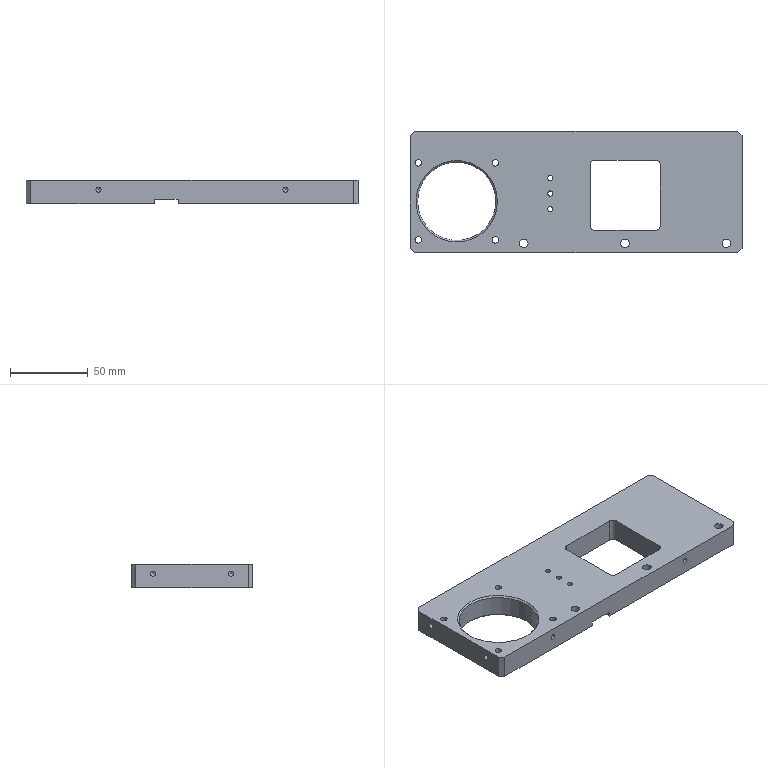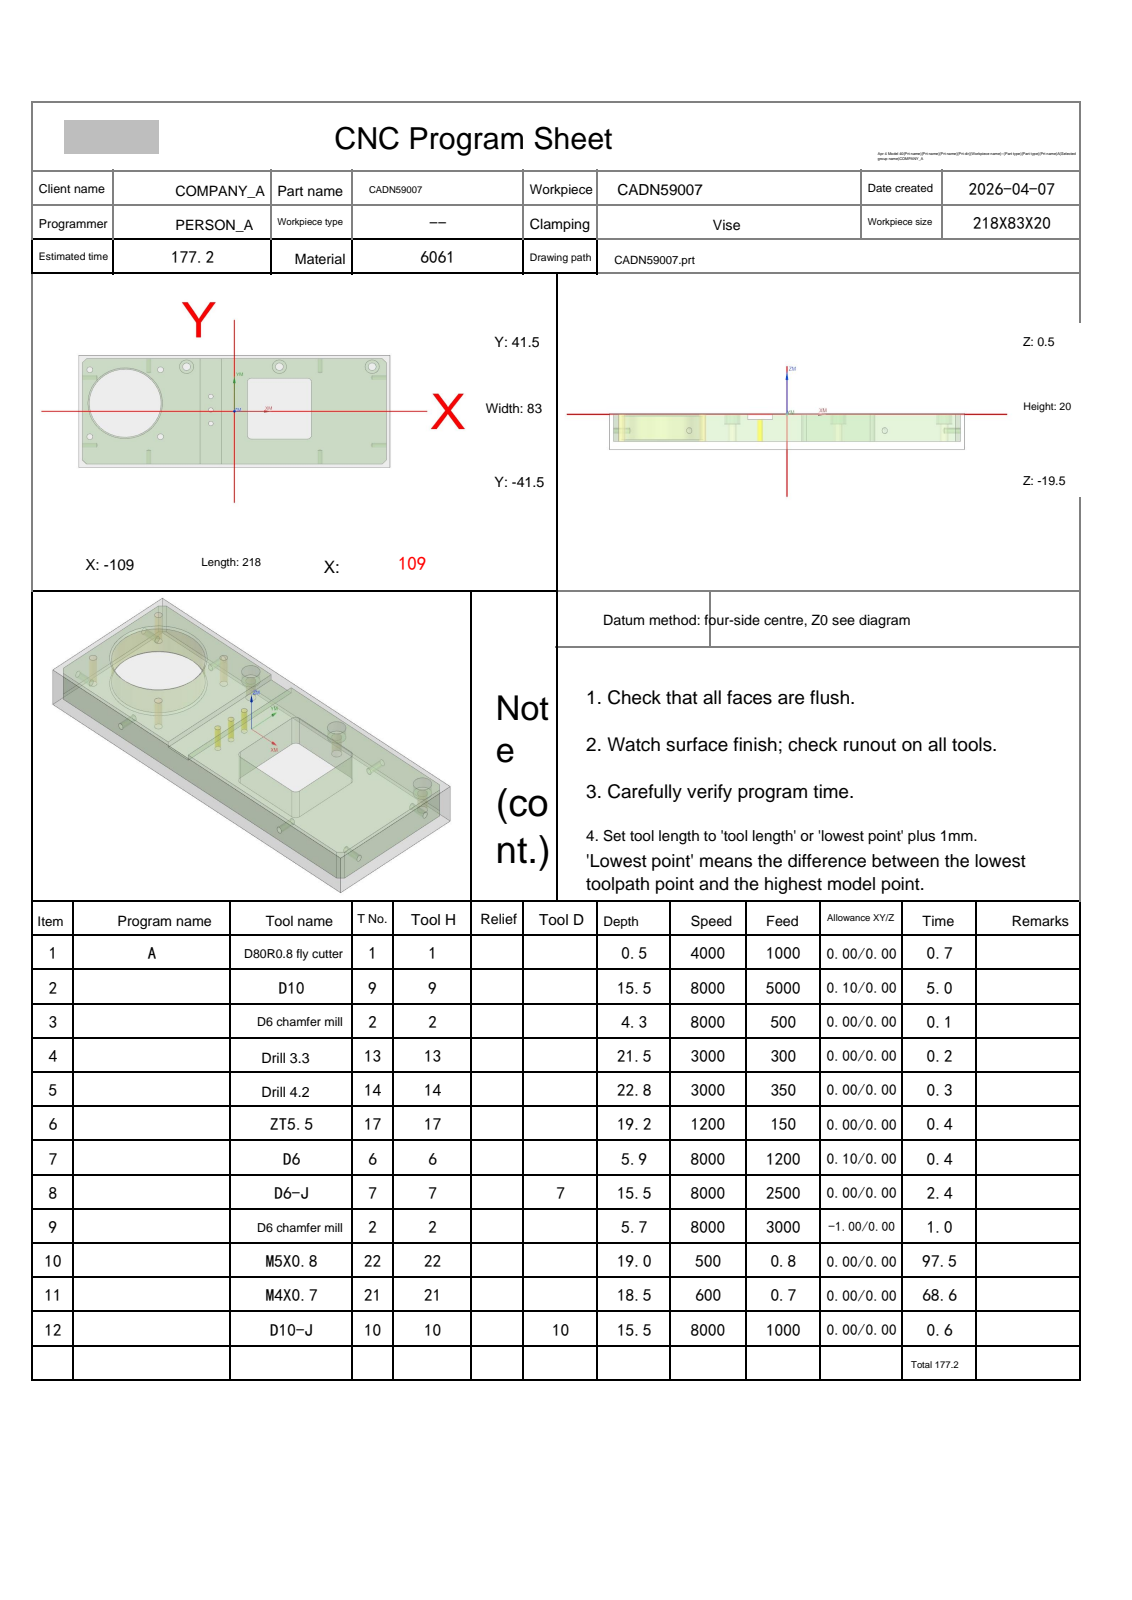NC program | NX | posted by the shop | part box 213 x 78 x 15 mm
Lines 1 to 890 of 7501:
%
O0001
(Machine time: 336.47 MIN)
(===Total Tool:11===)
(T1=D80R0.8 fly cutter D=80.  R=0.8  D-  H01 Z=0.    )
(T9=D10     D=10.  R=0.   D-  H09 Z=-15.  )
(T2=D6 chamfer mill   D=6.   R=0.   D-  H02 Z=-5.2  )
(T13=Drill 3.3  D=3.3  DR_a=118 D-  H13 Z=-20.99)
(T14=Drill 4.2  D=4.2  DR_a=118 D-  H14 Z=-22.26)
(T17=ZT5.5  D=5.5  DR_a=118 D-  H17 Z=-18.65)
(T6=D6      D=6.   R=0.   D-  H06 Z=-5.4  )
(T7=D6-J    D=6.   R=0.   D7  H07 Z=-15.  )
(T22=M5X0.8 D=4.2  DR_a=180 D-  H22 Z=-18.5 )
(T21=M4X0.7 D=3.3  DR_a=180 D-  H21 Z=-18.  )
(T10=D10-J  D=10.  R=0.   D10 H10 Z=-15.  )
G80 G90 G17 G49 G40
G91 G28 Z0
M01
N1 T01 M06
(D80R0.8 fly cutter  D=80. R=0.8 H=01 ce=0.00 di=0.00)
G00 G90 G54 X151.5 Y-26.333 M03 S4000
G43 H01 Z20.
M08
Z2.
G01 Z0.0 F1000.
X146.5
X-146.5
Y26.333
X146.5
X151.5
Z2.
G00 Z20.
G91 G28 Z0.0
M05
M09
G91 G28 Z0.0
M01
N2 T09 M06
(D10  D=10. R=0. H=09 ce=0.10 di=0.00)
G00 G90 G54 X0.0 Y44.1 M03 S8000
G43 H09 Z20.
M08
Z.5
G01 X103.5 Z.368 F5000.
G02 X107.106 Y42.606 Z.363 I0.0 J-5.1
G01 X110.106 Y39.606 Z.357
G02 X111.6 Y36. Z.352 I-3.606 J-3.606
G01 Y-36. Z.26
G02 X110.106 Y-39.606 Z.255 I-5.1 J0.0
G01 X107.106 Y-42.606 Z.25
G02 X103.5 Y-44.1 Z.245 I-3.606 J3.606
G01 X-103.5 Z-.02
G02 X-107.106 Y-42.606 Z-.025 I0.0 J5.1
G01 X-110.106 Y-39.606 Z-.03
G02 X-111.6 Y-36. Z-.035 I3.606 J3.606
G01 Y36. Z-.127
G02 X-110.106 Y39.606 Z-.132 I5.1 J0.0
G01 X-107.106 Y42.606 Z-.138
G02 X-103.5 Y44.1 Z-.143 I3.606 J-3.606
G01 X103.5 Z-.407
G02 X107.106 Y42.606 Z-.412 I0.0 J-5.1
G01 X110.106 Y39.606 Z-.418
G02 X111.6 Y36. Z-.423 I-3.606 J-3.606
G01 Y-36. Z-.515
G02 X110.106 Y-39.606 Z-.52 I-5.1 J0.0
G01 X107.106 Y-42.606 Z-.525
G02 X103.5 Y-44.1 Z-.53 I-3.606 J3.606
G01 X-103.5 Z-.795
G02 X-107.106 Y-42.606 Z-.8 I0.0 J5.1
G01 X-110.106 Y-39.606 Z-.805
G02 X-111.6 Y-36. Z-.81 I3.606 J3.606
G01 Y36. Z-.902
G02 X-110.106 Y39.606 Z-.907 I5.1 J0.0
G01 X-107.106 Y42.606 Z-.913
G02 X-103.5 Y44.1 Z-.918 I3.606 J-3.606
G01 X103.5 Z-1.182
G02 X107.106 Y42.606 Z-1.187 I0.0 J-5.1
G01 X110.106 Y39.606 Z-1.193
G02 X111.6 Y36. Z-1.198 I-3.606 J-3.606
G01 Y-36. Z-1.29
G02 X110.106 Y-39.606 Z-1.295 I-5.1 J0.0
G01 X107.106 Y-42.606 Z-1.3
G02 X103.5 Y-44.1 Z-1.305 I-3.606 J3.606
G01 X-103.5 Z-1.57
G02 X-107.106 Y-42.606 Z-1.575 I0.0 J5.1
G01 X-110.106 Y-39.606 Z-1.58
G02 X-111.6 Y-36. Z-1.585 I3.606 J3.606
G01 Y36. Z-1.677
G02 X-110.106 Y39.606 Z-1.682 I5.1 J0.0
G01 X-107.106 Y42.606 Z-1.688
G02 X-103.5 Y44.1 Z-1.693 I3.606 J-3.606
G01 X103.5 Z-1.957
G02 X107.106 Y42.606 Z-1.962 I0.0 J-5.1
G01 X110.106 Y39.606 Z-1.968
G02 X111.6 Y36. Z-1.973 I-3.606 J-3.606
G01 Y-36. Z-2.065
G02 X110.106 Y-39.606 Z-2.07 I-5.1 J0.0
G01 X107.106 Y-42.606 Z-2.075
G02 X103.5 Y-44.1 Z-2.08 I-3.606 J3.606
G01 X-103.5 Z-2.345
G02 X-107.106 Y-42.606 Z-2.35 I0.0 J5.1
G01 X-110.106 Y-39.606 Z-2.355
G02 X-111.6 Y-36. Z-2.36 I3.606 J3.606
G01 Y36. Z-2.452
G02 X-110.106 Y39.606 Z-2.457 I5.1 J0.0
G01 X-107.106 Y42.606 Z-2.463
G02 X-103.5 Y44.1 Z-2.468 I3.606 J-3.606
G01 X103.5 Z-2.732
G02 X107.106 Y42.606 Z-2.737 I0.0 J-5.1
G01 X110.106 Y39.606 Z-2.743
G02 X111.6 Y36. Z-2.748 I-3.606 J-3.606
G01 Y-36. Z-2.84
G02 X110.106 Y-39.606 Z-2.845 I-5.1 J0.0
G01 X107.106 Y-42.606 Z-2.85
G02 X103.5 Y-44.1 Z-2.855 I-3.606 J3.606
G01 X-103.5 Z-3.12
G02 X-107.106 Y-42.606 Z-3.125 I0.0 J5.1
G01 X-110.106 Y-39.606 Z-3.13
G02 X-111.6 Y-36. Z-3.135 I3.606 J3.606
G01 Y36. Z-3.227
G02 X-110.106 Y39.606 Z-3.232 I5.1 J0.0
G01 X-107.106 Y42.606 Z-3.238
G02 X-103.5 Y44.1 Z-3.243 I3.606 J-3.606
G01 X103.5 Z-3.507
G02 X107.106 Y42.606 Z-3.512 I0.0 J-5.1
G01 X110.106 Y39.606 Z-3.518
G02 X111.6 Y36. Z-3.523 I-3.606 J-3.606
G01 Y-36. Z-3.615
G02 X110.106 Y-39.606 Z-3.62 I-5.1 J0.0
G01 X107.106 Y-42.606 Z-3.625
G02 X103.5 Y-44.1 Z-3.63 I-3.606 J3.606
G01 X-103.5 Z-3.895
G02 X-107.106 Y-42.606 Z-3.9 I0.0 J5.1
G01 X-110.106 Y-39.606 Z-3.905
G02 X-111.6 Y-36. Z-3.91 I3.606 J3.606
G01 Y36. Z-4.002
G02 X-110.106 Y39.606 Z-4.007 I5.1 J0.0
G01 X-107.106 Y42.606 Z-4.013
G02 X-103.5 Y44.1 Z-4.018 I3.606 J-3.606
G01 X103.5 Z-4.282
G02 X107.106 Y42.606 Z-4.287 I0.0 J-5.1
G01 X110.106 Y39.606 Z-4.293
G02 X111.6 Y36. Z-4.298 I-3.606 J-3.606
G01 Y-36. Z-4.39
G02 X110.106 Y-39.606 Z-4.395 I-5.1 J0.0
G01 X107.106 Y-42.606 Z-4.4
G02 X103.5 Y-44.1 Z-4.405 I-3.606 J3.606
G01 X-103.5 Z-4.67
G02 X-107.106 Y-42.606 Z-4.675 I0.0 J5.1
G01 X-110.106 Y-39.606 Z-4.68
G02 X-111.6 Y-36. Z-4.685 I3.606 J3.606
G01 Y36. Z-4.777
G02 X-110.106 Y39.606 Z-4.782 I5.1 J0.0
G01 X-107.106 Y42.606 Z-4.788
G02 X-103.5 Y44.1 Z-4.793 I3.606 J-3.606
G01 X103.5 Z-5.057
G02 X107.106 Y42.606 Z-5.062 I0.0 J-5.1
G01 X110.106 Y39.606 Z-5.068
G02 X111.6 Y36. Z-5.073 I-3.606 J-3.606
G01 Y-36. Z-5.165
G02 X110.106 Y-39.606 Z-5.17 I-5.1 J0.0
G01 X107.106 Y-42.606 Z-5.175
G02 X103.5 Y-44.1 Z-5.18 I-3.606 J3.606
G01 X-103.5 Z-5.445
G02 X-107.106 Y-42.606 Z-5.45 I0.0 J5.1
G01 X-110.106 Y-39.606 Z-5.455
G02 X-111.6 Y-36. Z-5.46 I3.606 J3.606
G01 Y36. Z-5.552
G02 X-110.106 Y39.606 Z-5.557 I5.1 J0.0
G01 X-107.106 Y42.606 Z-5.563
G02 X-103.5 Y44.1 Z-5.568 I3.606 J-3.606
G01 X103.5 Z-5.832
G02 X107.106 Y42.606 Z-5.837 I0.0 J-5.1
G01 X110.106 Y39.606 Z-5.843
G02 X111.6 Y36. Z-5.848 I-3.606 J-3.606
G01 Y-36. Z-5.94
G02 X110.106 Y-39.606 Z-5.945 I-5.1 J0.0
G01 X107.106 Y-42.606 Z-5.95
G02 X103.5 Y-44.1 Z-5.955 I-3.606 J3.606
G01 X-103.5 Z-6.22
G02 X-107.106 Y-42.606 Z-6.225 I0.0 J5.1
G01 X-110.106 Y-39.606 Z-6.23
G02 X-111.6 Y-36. Z-6.235 I3.606 J3.606
G01 Y36. Z-6.327
G02 X-110.106 Y39.606 Z-6.332 I5.1 J0.0
G01 X-107.106 Y42.606 Z-6.338
G02 X-103.5 Y44.1 Z-6.343 I3.606 J-3.606
G01 X103.5 Z-6.607
G02 X107.106 Y42.606 Z-6.612 I0.0 J-5.1
G01 X110.106 Y39.606 Z-6.618
G02 X111.6 Y36. Z-6.623 I-3.606 J-3.606
G01 Y-36. Z-6.715
G02 X110.106 Y-39.606 Z-6.72 I-5.1 J0.0
G01 X107.106 Y-42.606 Z-6.725
G02 X103.5 Y-44.1 Z-6.73 I-3.606 J3.606
G01 X-103.5 Z-6.995
G02 X-107.106 Y-42.606 Z-7. I0.0 J5.1
G01 X-110.106 Y-39.606 Z-7.005
G02 X-111.6 Y-36. Z-7.01 I3.606 J3.606
G01 Y36. Z-7.102
G02 X-110.106 Y39.606 Z-7.107 I5.1 J0.0
G01 X-107.106 Y42.606 Z-7.113
G02 X-103.5 Y44.1 Z-7.118 I3.606 J-3.606
G01 X103.5 Z-7.382
G02 X107.106 Y42.606 Z-7.387 I0.0 J-5.1
G01 X110.106 Y39.606 Z-7.393
G02 X111.6 Y36. Z-7.398 I-3.606 J-3.606
G01 Y-36. Z-7.49
G02 X110.106 Y-39.606 Z-7.495 I-5.1 J0.0
G01 X107.106 Y-42.606 Z-7.5
G02 X103.5 Y-44.1 Z-7.505 I-3.606 J3.606
G01 X-103.5 Z-7.77
G02 X-107.106 Y-42.606 Z-7.775 I0.0 J5.1
G01 X-110.106 Y-39.606 Z-7.78
G02 X-111.6 Y-36. Z-7.785 I3.606 J3.606
G01 Y36. Z-7.877
G02 X-110.106 Y39.606 Z-7.882 I5.1 J0.0
G01 X-107.106 Y42.606 Z-7.888
G02 X-103.5 Y44.1 Z-7.893 I3.606 J-3.606
G01 X103.5 Z-8.157
G02 X107.106 Y42.606 Z-8.162 I0.0 J-5.1
G01 X110.106 Y39.606 Z-8.168
G02 X111.6 Y36. Z-8.173 I-3.606 J-3.606
G01 Y-36. Z-8.265
G02 X110.106 Y-39.606 Z-8.27 I-5.1 J0.0
G01 X107.106 Y-42.606 Z-8.275
G02 X103.5 Y-44.1 Z-8.28 I-3.606 J3.606
G01 X-103.5 Z-8.545
G02 X-107.106 Y-42.606 Z-8.55 I0.0 J5.1
G01 X-110.106 Y-39.606 Z-8.555
G02 X-111.6 Y-36. Z-8.56 I3.606 J3.606
G01 Y36. Z-8.652
G02 X-110.106 Y39.606 Z-8.657 I5.1 J0.0
G01 X-107.106 Y42.606 Z-8.663
G02 X-103.5 Y44.1 Z-8.668 I3.606 J-3.606
G01 X103.5 Z-8.932
G02 X107.106 Y42.606 Z-8.937 I0.0 J-5.1
G01 X110.106 Y39.606 Z-8.943
G02 X111.6 Y36. Z-8.948 I-3.606 J-3.606
G01 Y-36. Z-9.04
G02 X110.106 Y-39.606 Z-9.045 I-5.1 J0.0
G01 X107.106 Y-42.606 Z-9.05
G02 X103.5 Y-44.1 Z-9.055 I-3.606 J3.606
G01 X-103.5 Z-9.32
G02 X-107.106 Y-42.606 Z-9.325 I0.0 J5.1
G01 X-110.106 Y-39.606 Z-9.33
G02 X-111.6 Y-36. Z-9.335 I3.606 J3.606
G01 Y36. Z-9.427
G02 X-110.106 Y39.606 Z-9.432 I5.1 J0.0
G01 X-107.106 Y42.606 Z-9.438
G02 X-103.5 Y44.1 Z-9.443 I3.606 J-3.606
G01 X103.5 Z-9.707
G02 X107.106 Y42.606 Z-9.712 I0.0 J-5.1
G01 X110.106 Y39.606 Z-9.718
G02 X111.6 Y36. Z-9.723 I-3.606 J-3.606
G01 Y-36. Z-9.815
G02 X110.106 Y-39.606 Z-9.82 I-5.1 J0.0
G01 X107.106 Y-42.606 Z-9.825
G02 X103.5 Y-44.1 Z-9.83 I-3.606 J3.606
G01 X-103.5 Z-10.095
G02 X-107.106 Y-42.606 Z-10.1 I0.0 J5.1
G01 X-110.106 Y-39.606 Z-10.105
G02 X-111.6 Y-36. Z-10.11 I3.606 J3.606
G01 Y36. Z-10.202
G02 X-110.106 Y39.606 Z-10.207 I5.1 J0.0
G01 X-107.106 Y42.606 Z-10.213
G02 X-103.5 Y44.1 Z-10.218 I3.606 J-3.606
G01 X103.5 Z-10.482
G02 X107.106 Y42.606 Z-10.487 I0.0 J-5.1
G01 X110.106 Y39.606 Z-10.493
G02 X111.6 Y36. Z-10.498 I-3.606 J-3.606
G01 Y-36. Z-10.59
G02 X110.106 Y-39.606 Z-10.595 I-5.1 J0.0
G01 X107.106 Y-42.606 Z-10.6
G02 X103.5 Y-44.1 Z-10.605 I-3.606 J3.606
G01 X-103.5 Z-10.87
G02 X-107.106 Y-42.606 Z-10.875 I0.0 J5.1
G01 X-110.106 Y-39.606 Z-10.88
G02 X-111.6 Y-36. Z-10.885 I3.606 J3.606
G01 Y36. Z-10.977
G02 X-110.106 Y39.606 Z-10.982 I5.1 J0.0
G01 X-107.106 Y42.606 Z-10.988
G02 X-103.5 Y44.1 Z-10.993 I3.606 J-3.606
G01 X103.5 Z-11.257
G02 X107.106 Y42.606 Z-11.262 I0.0 J-5.1
G01 X110.106 Y39.606 Z-11.268
G02 X111.6 Y36. Z-11.273 I-3.606 J-3.606
G01 Y-36. Z-11.365
G02 X110.106 Y-39.606 Z-11.37 I-5.1 J0.0
G01 X107.106 Y-42.606 Z-11.375
G02 X103.5 Y-44.1 Z-11.38 I-3.606 J3.606
G01 X-103.5 Z-11.645
G02 X-107.106 Y-42.606 Z-11.65 I0.0 J5.1
G01 X-110.106 Y-39.606 Z-11.655
G02 X-111.6 Y-36. Z-11.66 I3.606 J3.606
G01 Y36. Z-11.752
G02 X-110.106 Y39.606 Z-11.757 I5.1 J0.0
G01 X-107.106 Y42.606 Z-11.763
G02 X-103.5 Y44.1 Z-11.768 I3.606 J-3.606
G01 X103.5 Z-12.032
G02 X107.106 Y42.606 Z-12.037 I0.0 J-5.1
G01 X110.106 Y39.606 Z-12.043
G02 X111.6 Y36. Z-12.048 I-3.606 J-3.606
G01 Y-36. Z-12.14
G02 X110.106 Y-39.606 Z-12.145 I-5.1 J0.0
G01 X107.106 Y-42.606 Z-12.15
G02 X103.5 Y-44.1 Z-12.155 I-3.606 J3.606
G01 X-103.5 Z-12.42
G02 X-107.106 Y-42.606 Z-12.425 I0.0 J5.1
G01 X-110.106 Y-39.606 Z-12.43
G02 X-111.6 Y-36. Z-12.435 I3.606 J3.606
G01 Y36. Z-12.527
G02 X-110.106 Y39.606 Z-12.532 I5.1 J0.0
G01 X-107.106 Y42.606 Z-12.538
G02 X-103.5 Y44.1 Z-12.543 I3.606 J-3.606
G01 X103.5 Z-12.807
G02 X107.106 Y42.606 Z-12.812 I0.0 J-5.1
G01 X110.106 Y39.606 Z-12.818
G02 X111.6 Y36. Z-12.823 I-3.606 J-3.606
G01 Y-36. Z-12.915
G02 X110.106 Y-39.606 Z-12.92 I-5.1 J0.0
G01 X107.106 Y-42.606 Z-12.925
G02 X103.5 Y-44.1 Z-12.93 I-3.606 J3.606
G01 X-103.5 Z-13.195
G02 X-107.106 Y-42.606 Z-13.2 I0.0 J5.1
G01 X-110.106 Y-39.606 Z-13.205
G02 X-111.6 Y-36. Z-13.21 I3.606 J3.606
G01 Y36. Z-13.302
G02 X-110.106 Y39.606 Z-13.307 I5.1 J0.0
G01 X-107.106 Y42.606 Z-13.313
G02 X-103.5 Y44.1 Z-13.318 I3.606 J-3.606
G01 X103.5 Z-13.582
G02 X107.106 Y42.606 Z-13.587 I0.0 J-5.1
G01 X110.106 Y39.606 Z-13.593
G02 X111.6 Y36. Z-13.598 I-3.606 J-3.606
G01 Y-36. Z-13.69
G02 X110.106 Y-39.606 Z-13.695 I-5.1 J0.0
G01 X107.106 Y-42.606 Z-13.7
G02 X103.5 Y-44.1 Z-13.705 I-3.606 J3.606
G01 X-103.5 Z-13.97
G02 X-107.106 Y-42.606 Z-13.975 I0.0 J5.1
G01 X-110.106 Y-39.606 Z-13.98
G02 X-111.6 Y-36. Z-13.985 I3.606 J3.606
G01 Y36. Z-14.077
G02 X-110.106 Y39.606 Z-14.082 I5.1 J0.0
G01 X-107.106 Y42.606 Z-14.088
G02 X-103.5 Y44.1 Z-14.093 I3.606 J-3.606
G01 X103.5 Z-14.357
G02 X107.106 Y42.606 Z-14.362 I0.0 J-5.1
G01 X110.106 Y39.606 Z-14.368
G02 X111.6 Y36. Z-14.373 I-3.606 J-3.606
G01 Y-36. Z-14.465
G02 X110.106 Y-39.606 Z-14.47 I-5.1 J0.0
G01 X107.106 Y-42.606 Z-14.475
G02 X103.5 Y-44.1 Z-14.48 I-3.606 J3.606
G01 X-103.5 Z-14.745
G02 X-107.106 Y-42.606 Z-14.75 I0.0 J5.1
G01 X-110.106 Y-39.606 Z-14.755
G02 X-111.6 Y-36. Z-14.76 I3.606 J3.606
G01 Y36. Z-14.852
G02 X-110.106 Y39.606 Z-14.857 I5.1 J0.0
G01 X-107.106 Y42.606 Z-14.863
G02 X-103.5 Y44.1 Z-14.868 I3.606 J-3.606
G01 X0.0 Z-15.
X103.5
G02 X107.106 Y42.606 I0.0 J-5.1
G01 X110.106 Y39.606
G02 X111.6 Y36. I-3.606 J-3.606
G01 Y-36.
G02 X110.106 Y-39.606 I-5.1 J0.0
G01 X107.106 Y-42.606
G02 X103.5 Y-44.1 I-3.606 J3.606
G01 X-103.5
G02 X-107.106 Y-42.606 I0.0 J5.1
G01 X-110.106 Y-39.606
G02 X-111.6 Y-36. I3.606 J3.606
G01 Y36.
G02 X-110.106 Y39.606 I5.1 J0.0
G01 X-107.106 Y42.606
G02 X-103.5 Y44.1 I3.606 J-3.606
G01 X0.0
X.5
Z-14.
G00 Z20.
G00 G90 X-16.5 Y47.1 M03 S6000
Z20.
Z.017
G01 Z-.483 F3500.
Y40.
X-18.95
Y-40.
X-14.05
Y40.
X-16.5
X-17.
Z.017
G00 Z.5
X-16.5 Y47.1
Z-.467
G01 Z-.967
Y40.
X-18.95
Y-40.
X-14.05
Y40.
X-16.5
X-17.
Z-.467
G00 Z.017
X-16.5 Y47.1
Z-.95
G01 Z-1.45
Y40.
X-18.95
Y-40.
X-14.05
Y40.
X-16.5
X-17.
Z-.95
G00 Z-.467
X-16.5 Y47.1
Z-1.433
G01 Z-1.933
Y40.
X-18.95
Y-40.
X-14.05
Y40.
X-16.5
X-17.
Z-1.433
G00 Z-.95
X-16.5 Y47.1
Z-1.917
G01 Z-2.417
Y40.
X-18.95
Y-40.
X-14.05
Y40.
X-16.5
X-17.
Z-1.917
G00 Z-1.433
X-16.5 Y47.1
Z-2.4
G01 Z-2.9
Y40.
X-18.95
Y-40.
X-14.05
Y40.
X-16.5
X-17.
Z-2.4
G00 Z20.
G00 G90 X31.5 Y19.4 M03 S6000
Z20.
Z.5
G01 X14.1 Z.438 F4000.
Y-15.4 Z.315
X48.9 Z.192
Y19.4 Z.068
X14.1 Z-.055
Y-15.4 Z-.179
X48.9 Z-.302
Y19.4 Z-.425
X14.1 Z-.549
Y-15.4 Z-.672
X48.9 Z-.796
Y19.4 Z-.919
X14.1 Z-1.042
Y-15.4 Z-1.166
X48.9 Z-1.289
Y19.4 Z-1.413
X14.1 Z-1.536
Y-15.4 Z-1.659
X48.9 Z-1.783
Y19.4 Z-1.906
X14.1 Z-2.029
Y-15.4 Z-2.153
X48.9 Z-2.276
Y19.4 Z-2.4
X14.1 Z-2.523
Y-15.4 Z-2.646
X48.9 Z-2.77
Y19.4 Z-2.893
X14.1 Z-3.017
Y-15.4 Z-3.14
X48.9 Z-3.263
Y19.4 Z-3.387
X14.1 Z-3.51
Y-15.4 Z-3.633
X48.9 Z-3.757
Y19.4 Z-3.88
X14.1 Z-4.004
Y-15.4 Z-4.127
X48.9 Z-4.25
Y19.4 Z-4.374
X14.1 Z-4.497
Y-15.4 Z-4.621
X48.9 Z-4.744
Y19.4 Z-4.867
X14.1 Z-4.991
Y-15.4 Z-5.114
X48.9 Z-5.238
Y19.4 Z-5.361
X14.1 Z-5.484
Y-15.4 Z-5.608
X48.9 Z-5.731
Y19.4 Z-5.854
X14.1 Z-5.978
Y-15.4 Z-6.101
X48.9 Z-6.225
Y19.4 Z-6.348
X14.1 Z-6.471
Y-15.4 Z-6.595
X48.9 Z-6.718
Y19.4 Z-6.842
X14.1 Z-6.965
Y-15.4 Z-7.088
X48.9 Z-7.212
Y19.4 Z-7.335
X14.1 Z-7.458
Y-15.4 Z-7.582
X48.9 Z-7.705
Y19.4 Z-7.829
X14.1 Z-7.952
Y-15.4 Z-8.075
X48.9 Z-8.199
Y19.4 Z-8.322
X14.1 Z-8.446
Y-15.4 Z-8.569
X48.9 Z-8.692
Y19.4 Z-8.816
X14.1 Z-8.939
Y-15.4 Z-9.063
X48.9 Z-9.186
Y19.4 Z-9.309
X14.1 Z-9.433
Y-15.4 Z-9.556
X48.9 Z-9.679
Y19.4 Z-9.803
X14.1 Z-9.926
Y-15.4 Z-10.05
X48.9 Z-10.173
Y19.4 Z-10.296
X14.1 Z-10.42
Y-15.4 Z-10.543
X48.9 Z-10.667
Y19.4 Z-10.79
X14.1 Z-10.913
Y-15.4 Z-11.037
X48.9 Z-11.16
Y19.4 Z-11.283
X14.1 Z-11.407
Y-15.4 Z-11.53
X48.9 Z-11.654
Y19.4 Z-11.777
X14.1 Z-11.9
Y-15.4 Z-12.024
X48.9 Z-12.147
Y19.4 Z-12.271
X14.1 Z-12.394
Y-15.4 Z-12.517
X48.9 Z-12.641
Y19.4 Z-12.764
X14.1 Z-12.888
Y-15.4 Z-13.011
X48.9 Z-13.134
Y19.4 Z-13.258
X14.1 Z-13.381
Y-15.4 Z-13.504
X48.9 Z-13.628
Y19.4 Z-13.751
X14.1 Z-13.875
Y-15.4 Z-13.998
X48.9 Z-14.121
Y19.4 Z-14.245
X14.1 Z-14.368
Y-15.4 Z-14.492
X48.9 Z-14.615
Y19.4 Z-14.738
X31.5 Z-14.8
X14.1
Y-15.4
X48.9
Y19.4
X31.5
X31.
Z-13.8
G00 Z20.
X-76.5 Y26.05
Z.5
G03 X-96.55 Y6. Z.377 I0.0 J-20.05
X-76.5 Y-14.05 Z.253 I20.05 J0.0
X-56.45 Y6. Z.13 I0.0 J20.05
X-76.5 Y26.05 Z.006 I-20.05 J0.0
X-96.55 Y6. Z-.117 I0.0 J-20.05
X-76.5 Y-14.05 Z-.24 I20.05 J0.0
X-56.45 Y6. Z-.364 I0.0 J20.05
X-76.5 Y26.05 Z-.487 I-20.05 J0.0
X-96.55 Y6. Z-.61 I0.0 J-20.05
X-76.5 Y-14.05 Z-.734 I20.05 J0.0
X-56.45 Y6. Z-.857 I0.0 J20.05
X-76.5 Y26.05 Z-.981 I-20.05 J0.0
X-96.55 Y6. Z-1.104 I0.0 J-20.05
X-76.5 Y-14.05 Z-1.227 I20.05 J0.0
X-56.45 Y6. Z-1.351 I0.0 J20.05
X-76.5 Y26.05 Z-1.474 I-20.05 J0.0
X-96.55 Y6. Z-1.598 I0.0 J-20.05
X-76.5 Y-14.05 Z-1.721 I20.05 J0.0
X-56.45 Y6. Z-1.844 I0.0 J20.05
X-76.5 Y26.05 Z-1.968 I-20.05 J0.0
X-96.55 Y6. Z-2.091 I0.0 J-20.05
X-76.5 Y-14.05 Z-2.215 I20.05 J0.0
X-56.45 Y6. Z-2.338 I0.0 J20.05
X-76.5 Y26.05 Z-2.461 I-20.05 J0.0
X-96.55 Y6. Z-2.585 I0.0 J-20.05
X-76.5 Y-14.05 Z-2.708 I20.05 J0.0
X-56.45 Y6. Z-2.831 I0.0 J20.05
X-76.5 Y26.05 Z-2.955 I-20.05 J0.0
X-96.55 Y6. Z-3.078 I0.0 J-20.05
X-76.5 Y-14.05 Z-3.202 I20.05 J0.0
X-56.45 Y6. Z-3.325 I0.0 J20.05
X-76.5 Y26.05 Z-3.448 I-20.05 J0.0
X-96.55 Y6. Z-3.572 I0.0 J-20.05
X-76.5 Y-14.05 Z-3.695 I20.05 J0.0
X-56.45 Y6. Z-3.819 I0.0 J20.05
X-76.5 Y26.05 Z-3.942 I-20.05 J0.0
X-96.55 Y6. Z-4.065 I0.0 J-20.05
X-76.5 Y-14.05 Z-4.189 I20.05 J0.0
X-56.45 Y6. Z-4.312 I0.0 J20.05
X-76.5 Y26.05 Z-4.435 I-20.05 J0.0
X-96.55 Y6. Z-4.559 I0.0 J-20.05
X-76.5 Y-14.05 Z-4.682 I20.05 J0.0
X-56.45 Y6. Z-4.806 I0.0 J20.05
X-76.5 Y26.05 Z-4.929 I-20.05 J0.0
X-96.55 Y6. Z-5.052 I0.0 J-20.05
X-76.5 Y-14.05 Z-5.176 I20.05 J0.0
X-56.45 Y6. Z-5.299 I0.0 J20.05
X-76.5 Y26.05 Z-5.423 I-20.05 J0.0
X-96.55 Y6. Z-5.546 I0.0 J-20.05
X-76.5 Y-14.05 Z-5.669 I20.05 J0.0
X-56.45 Y6. Z-5.793 I0.0 J20.05
X-76.5 Y26.05 Z-5.916 I-20.05 J0.0
X-96.55 Y6. Z-6.04 I0.0 J-20.05
X-76.5 Y-14.05 Z-6.163 I20.05 J0.0
X-56.45 Y6. Z-6.286 I0.0 J20.05
X-76.5 Y26.05 Z-6.41 I-20.05 J0.0
X-96.55 Y6. Z-6.533 I0.0 J-20.05
X-76.5 Y-14.05 Z-6.656 I20.05 J0.0
X-56.45 Y6. Z-6.78 I0.0 J20.05
X-76.5 Y26.05 Z-6.903 I-20.05 J0.0
X-96.55 Y6. Z-7.027 I0.0 J-20.05
X-76.5 Y-14.05 Z-7.15 I20.05 J0.0
X-56.45 Y6. Z-7.273 I0.0 J20.05
X-76.5 Y26.05 Z-7.397 I-20.05 J0.0
X-96.55 Y6. Z-7.52 I0.0 J-20.05
X-76.5 Y-14.05 Z-7.644 I20.05 J0.0
X-56.45 Y6. Z-7.767 I0.0 J20.05
X-76.5 Y26.05 Z-7.89 I-20.05 J0.0
X-96.55 Y6. Z-8.014 I0.0 J-20.05
X-76.5 Y-14.05 Z-8.137 I20.05 J0.0
X-56.45 Y6. Z-8.26 I0.0 J20.05
X-76.5 Y26.05 Z-8.384 I-20.05 J0.0
X-96.55 Y6. Z-8.507 I0.0 J-20.05
X-76.5 Y-14.05 Z-8.631 I20.05 J0.0
X-56.45 Y6. Z-8.754 I0.0 J20.05
X-76.5 Y26.05 Z-8.877 I-20.05 J0.0
X-96.55 Y6. Z-9.001 I0.0 J-20.05
X-76.5 Y-14.05 Z-9.124 I20.05 J0.0
X-56.45 Y6. Z-9.248 I0.0 J20.05
X-76.5 Y26.05 Z-9.371 I-20.05 J0.0
X-96.55 Y6. Z-9.494 I0.0 J-20.05
X-76.5 Y-14.05 Z-9.618 I20.05 J0.0
X-56.45 Y6. Z-9.741 I0.0 J20.05
X-76.5 Y26.05 Z-9.865 I-20.05 J0.0
X-96.55 Y6. Z-9.988 I0.0 J-20.05
X-76.5 Y-14.05 Z-10.111 I20.05 J0.0
X-56.45 Y6. Z-10.235 I0.0 J20.05
X-76.5 Y26.05 Z-10.358 I-20.05 J0.0
X-96.55 Y6. Z-10.481 I0.0 J-20.05
X-76.5 Y-14.05 Z-10.605 I20.05 J0.0
X-56.45 Y6. Z-10.728 I0.0 J20.05
X-76.5 Y26.05 Z-10.852 I-20.05 J0.0
X-96.55 Y6. Z-10.975 I0.0 J-20.05
X-76.5 Y-14.05 Z-11.098 I20.05 J0.0
X-56.45 Y6. Z-11.222 I0.0 J20.05
X-76.5 Y26.05 Z-11.345 I-20.05 J0.0
X-96.55 Y6. Z-11.469 I0.0 J-20.05
X-76.5 Y-14.05 Z-11.592 I20.05 J0.0
X-56.45 Y6. Z-11.715 I0.0 J20.05
X-76.5 Y26.05 Z-11.839 I-20.05 J0.0
X-96.55 Y6. Z-11.962 I0.0 J-20.05
X-76.5 Y-14.05 Z-12.085 I20.05 J0.0
X-56.45 Y6. Z-12.209 I0.0 J20.05
X-76.5 Y26.05 Z-12.332 I-20.05 J0.0
X-96.55 Y6. Z-12.456 I0.0 J-20.05
X-76.5 Y-14.05 Z-12.579 I20.05 J0.0
X-56.45 Y6. Z-12.702 I0.0 J20.05
X-76.5 Y26.05 Z-12.826 I-20.05 J0.0
X-96.55 Y6. Z-12.949 I0.0 J-20.05
X-76.5 Y-14.05 Z-13.073 I20.05 J0.0
X-56.45 Y6. Z-13.196 I0.0 J20.05
X-76.5 Y26.05 Z-13.319 I-20.05 J0.0
X-96.55 Y6. Z-13.443 I0.0 J-20.05
X-76.5 Y-14.05 Z-13.566 I20.05 J0.0
X-56.45 Y6. Z-13.69 I0.0 J20.05
X-76.5 Y26.05 Z-13.813 I-20.05 J0.0
X-96.55 Y6. Z-13.936 I0.0 J-20.05
X-76.5 Y-14.05 Z-14.06 I20.05 J0.0
X-56.45 Y6. Z-14.183 I0.0 J20.05
X-76.5 Y26.05 Z-14.306 I-20.05 J0.0
X-96.55 Y6. Z-14.43 I0.0 J-20.05
X-76.5 Y-14.05 Z-14.553 I20.05 J0.0
X-56.45 Y6. Z-14.677 I0.0 J20.05
X-76.5 Y26.05 Z-14.8 I-20.05 J0.0
X-96.55 Y6. I0.0 J-20.05
X-76.5 Y-14.05 I20.05 J0.0
X-56.45 Y6. I0.0 J20.05
X-76.5 Y26.05 I-20.05 J0.0
X-77. Y26.044 I0.0 J-20.05
G01 Z-13.8
G00 Z20.
G91 G28 Z0.0
M05
M09
G91 G28 Z0.0
M01
N3 T02 M06
(D6 chamfer mill  D=6. R=0. H=02 ce=0.00 di=0.00)
G00 G90 G54 X96.5 Y33. M03 S8000
G43 H02 Z20.
M08
G98 G81 X96.5 Y33. Z-.8 R1. F500.
X31.5
X-16.5 Y11. Z-3.8 R-2.
Y1.
Y-9.
X-51.751 Y-18.749 Z-.8 R1.
X-101.249
Y30.749
X-51.751
X-33.5 Y33.
G80
G00 Z20.
G00 G90 X-76.5 Y6. M03 S8000
Z20.
G98 G82 X-76.5 Y6. Z-.8 R1. F500.
G80
G00 Z20.
G91 G28 Z0.0
M05
M09
G91 G28 Z0.0
M01
N4 T13 M06
(Drill 3.3 D=3.3 DR_a=118 H=13)
G00 G90 G54 X-16.5 Y11. M03 S3000
G43 H13 Z20.
M08
G98 G83 X-16.5 Y11. Z-20.991 R-2. F300. Q2.
Y1.
Y-9.
G80
G00 Z20.
G91 G28 Z0.0
M05
M09
G91 G28 Z0.0
M01
N5 T14 M06
(Drill 4.2 D=4.2 DR_a=118 H=14)
G00 G90 G54 X-51.751 Y30.749 M03 S3000
G43 H14 Z20.
M08
G98 G83 X-51.751 Y30.749 Z-22.262 R1. F350. Q3.
X-101.249
Y-18.749
X-51.751
G80
G00 Z20.
G91 G28 Z0.0
M05
M09
G91 G28 Z0.0
M01
N6 T17 M06
(ZT5.5 D=5.5 DR_a=118 H=17)
G00 G90 G54 X96.5 Y33. M03 S1200
G43 H17 Z20.
M08
G98 G83 X96.5 Y33. Z-18.652 R1. F150. Q2.
X31.5
X-33.5
G80
G00 Z20.
G91 G28 Z0.0
M05
M09
G91 G28 Z0.0
M01
N7 T06 M06
(D6  D=6. R=0. H=06 ce=0.10 di=0.00)
G00 G90 G54 X31.5 Y33. M03 S8000
G43 H06 Z20.
M08
Z.5
G03 X32.45 Y32.05 I.95 J0.0 F1200.
X33.4 Y33. I0.0 J.95
X33.4 Y33. Z0.0 I-1.9 J0.0
X33.4 Y33. Z-.5 I-1.9 J0.0
X33.4 Y33. Z-1. I-1.9 J0.0
X33.4 Y33. Z-1.5 I-1.9 J0.0
X33.4 Y33. Z-2. I-1.9 J0.0
X33.4 Y33. Z-2.5 I-1.9 J0.0
X33.4 Y33. Z-3. I-1.9 J0.0
X33.4 Y33. Z-3.5 I-1.9 J0.0
X33.4 Y33. Z-4. I-1.9 J0.0
X33.4 Y33. Z-4.5 I-1.9 J0.0
X33.4 Y33. Z-5. I-1.9 J0.0
X32.087 Y31.193 Z-5.4 I-1.9 J0.0
X33.4 Y33. I-.587 J1.807
X31.5 Y34.9 I-1.9 J0.0
X29.6 Y33. I0.0 J-1.9
X31.5 Y31.1 I1.9 J0.0
X32.087 Y31.193 I0.0 J1.9
X32.744 Y32.096 I-.294 J.904
X31.794 Y33.046 I-.95 J0.0
X31.5 Y33. I0.0 J-.95
G00 Z20.
X96.5
Z.5
G03 X97.45 Y32.05 I.95 J0.0
X98.4 Y33. I0.0 J.95
X98.4 Y33. Z0.0 I-1.9 J0.0
X98.4 Y33. Z-.5 I-1.9 J0.0
X98.4 Y33. Z-1. I-1.9 J0.0
X98.4 Y33. Z-1.5 I-1.9 J0.0
X98.4 Y33. Z-2. I-1.9 J0.0
X98.4 Y33. Z-2.5 I-1.9 J0.0
X98.4 Y33. Z-3. I-1.9 J0.0
X98.4 Y33. Z-3.5 I-1.9 J0.0
X98.4 Y33. Z-4. I-1.9 J0.0
X98.4 Y33. Z-4.5 I-1.9 J0.0
X98.4 Y33. Z-5. I-1.9 J0.0
X97.087 Y31.193 Z-5.4 I-1.9 J0.0
X98.4 Y33. I-.587 J1.807
X96.5 Y34.9 I-1.9 J0.0
X94.6 Y33. I0.0 J-1.9
X96.5 Y31.1 I1.9 J0.0
X97.087 Y31.193 I0.0 J1.9
X97.744 Y32.096 I-.294 J.904
X96.794 Y33.046 I-.95 J0.0
X96.5 Y33. I0.0 J-.95
G00 Z20.
X-33.5
Z.5
G03 X-32.55 Y32.05 I.95 J0.0
X-31.6 Y33. I0.0 J.95
X-31.6 Y33. Z0.0 I-1.9 J0.0
X-31.6 Y33. Z-.5 I-1.9 J0.0
X-31.6 Y33. Z-1. I-1.9 J0.0
X-31.6 Y33. Z-1.5 I-1.9 J0.0
X-31.6 Y33. Z-2. I-1.9 J0.0
X-31.6 Y33. Z-2.5 I-1.9 J0.0
X-31.6 Y33. Z-3. I-1.9 J0.0
X-31.6 Y33. Z-3.5 I-1.9 J0.0
X-31.6 Y33. Z-4. I-1.9 J0.0
X-31.6 Y33. Z-4.5 I-1.9 J0.0
X-31.6 Y33. Z-5. I-1.9 J0.0
X-32.913 Y31.193 Z-5.4 I-1.9 J0.0
X-31.6 Y33. I-.587 J1.807
X-33.5 Y34.9 I-1.9 J0.0
X-35.4 Y33. I0.0 J-1.9
X-33.5 Y31.1 I1.9 J0.0
X-32.913 Y31.193 I0.0 J1.9
X-32.256 Y32.096 I-.294 J.904
X-33.206 Y33.046 I-.95 J0.0
X-33.5 Y33. I0.0 J-.95
G00 Z20.
G91 G28 Z0.0
M05
M09
G91 G28 Z0.0
M01